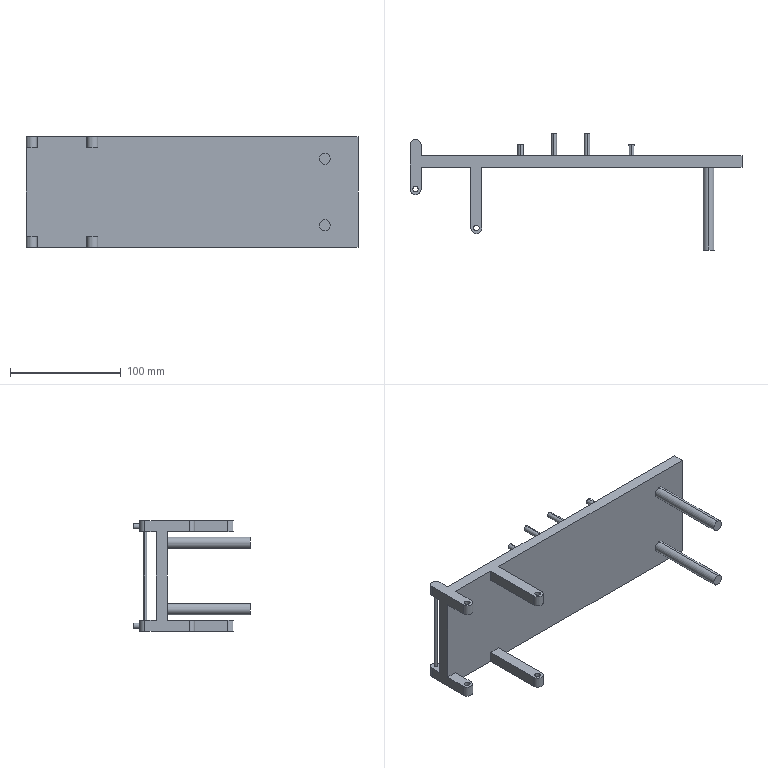Part | SolidWorks | features ICE 7, MirrorPattern 2, Extrusion 1, Fillet 1 | 1 solid | 68 faces | box 300 x 105 x 100 mm | volume 333273 mm3 | cylinder 38 | plane 30 | commonest cylinder face diameters 5 x24 10 x12 3 x2